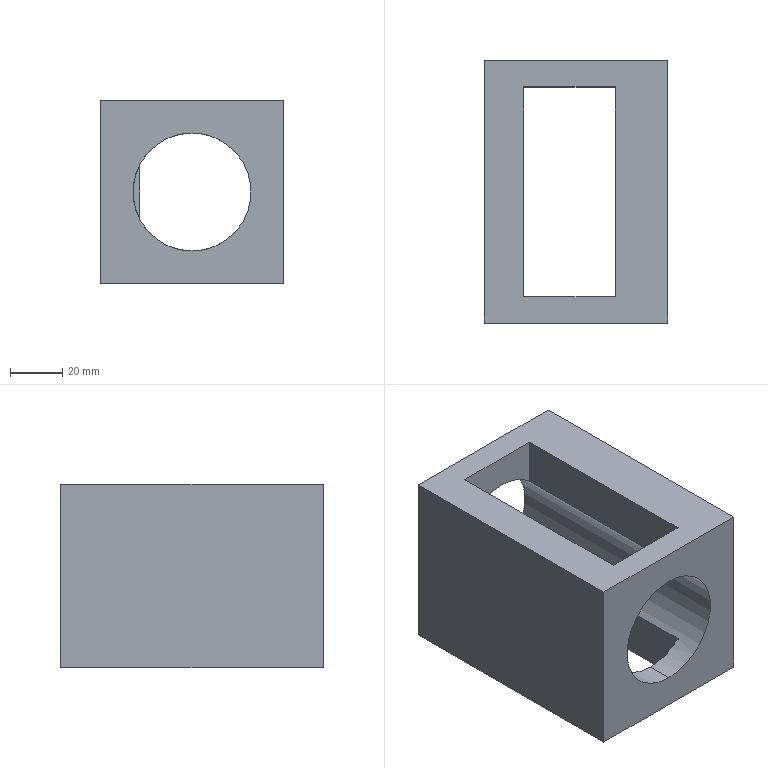Part | STEP file | Boss-Extrude 4 | 1 solid | 34 faces | box 70 x 100 x 70 mm | volume 247035 mm3 | plane 15 | cylinder 11 | cone 8 | commonest cylinder face diameters 5 x8 45 x3
STEP:
#1=CARTESIAN_POINT('',(-1518.738,1643.264,2784.251));
#2=VERTEX_POINT('',#1);
#3=CARTESIAN_POINT('',(-1518.738,1643.264,2789.251));
#4=VERTEX_POINT('',#3);
#5=CARTESIAN_POINT('',(-1518.738,1643.264,2786.751));
#6=DIRECTION('',(0.,1.,0.));
#7=DIRECTION('',(0.,0.,1.));
#8=AXIS2_PLACEMENT_3D('',#5,#6,#7);
#9=CIRCLE('',#8,2.5);
#10=EDGE_CURVE('',#2,#4,#9,.T.);
#11=ORIENTED_EDGE('',*,*,#10,.F.);
#12=CARTESIAN_POINT('',(-1518.738,1658.264,2784.251));
#13=VERTEX_POINT('',#12);
#14=CARTESIAN_POINT('',(-1518.738,1658.264,2784.251));
#15=DIRECTION('',(0.,1.,0.));
#16=VECTOR('',#15,1000.);
#17=LINE('',#14,#16);
#18=EDGE_CURVE('',#2,#13,#17,.T.);
#19=ORIENTED_EDGE('',*,*,#18,.T.);
#20=CARTESIAN_POINT('',(-1518.738,1658.264,2789.251));
#21=VERTEX_POINT('',#20);
#22=CARTESIAN_POINT('',(-1518.738,1658.264,2786.751));
#23=DIRECTION('',(0.,1.,0.));
#24=DIRECTION('',(0.,0.,1.));
#25=AXIS2_PLACEMENT_3D('',#22,#23,#24);
#26=CIRCLE('',#25,2.5);
#27=EDGE_CURVE('',#13,#21,#26,.T.);
#28=ORIENTED_EDGE('',*,*,#27,.T.);
#29=CARTESIAN_POINT('',(-1518.738,1658.264,2789.251));
#30=DIRECTION('',(0.,1.,0.));
#31=VECTOR('',#30,1000.);
#32=LINE('',#29,#31);
#33=EDGE_CURVE('',#4,#21,#32,.T.);
#34=ORIENTED_EDGE('',*,*,#33,.F.);
#35=EDGE_LOOP('',(#11,#19,#28,#34));
#36=FACE_OUTER_BOUND('',#35,.T.);
#37=CARTESIAN_POINT('',(-1518.738,1658.264,2786.751));
#38=DIRECTION('',(0.,1.,0.));
#39=DIRECTION('',(0.,0.,-1.));
#40=AXIS2_PLACEMENT_3D('',#37,#38,#39);
#41=CYLINDRICAL_SURFACE('',#40,2.5);
#42=ADVANCED_FACE('',(#36),#41,.F.);
#43=CARTESIAN_POINT('',(-1518.738,1641.762,2786.751));
#44=VERTEX_POINT('',#43);
#45=CARTESIAN_POINT('',(-1518.738,1643.264,2789.251));
#46=DIRECTION('',(0.,0.515,0.8572));
#47=VECTOR('',#46,1000.);
#48=LINE('',#45,#47);
#49=EDGE_CURVE('',#44,#4,#48,.T.);
#50=ORIENTED_EDGE('',*,*,#49,.F.);
#51=CARTESIAN_POINT('',(-1518.738,1643.264,2784.251));
#52=DIRECTION('',(0.,0.515,-0.8572));
#53=VECTOR('',#52,1000.);
#54=LINE('',#51,#53);
#55=EDGE_CURVE('',#44,#2,#54,.T.);
#56=ORIENTED_EDGE('',*,*,#55,.T.);
#57=ORIENTED_EDGE('',*,*,#10,.T.);
#58=EDGE_LOOP('',(#50,#56,#57));
#59=FACE_OUTER_BOUND('',#58,.T.);
#60=CARTESIAN_POINT('',(-1518.738,1643.264,2786.751));
#61=DIRECTION('',(0.,1.,0.));
#62=DIRECTION('',(0.,0.,-1.));
#63=AXIS2_PLACEMENT_3D('',#60,#61,#62);
#64=CONICAL_SURFACE('',#63,2.5,1.03);
#65=ADVANCED_FACE('',(#59),#64,.F.);
#66=CARTESIAN_POINT('',(-1458.738,1643.264,2844.251));
#67=VERTEX_POINT('',#66);
#68=CARTESIAN_POINT('',(-1458.738,1643.264,2849.251));
#69=VERTEX_POINT('',#68);
#70=CARTESIAN_POINT('',(-1458.738,1643.264,2846.751));
#71=DIRECTION('',(0.,1.,0.));
#72=DIRECTION('',(0.,0.,1.));
#73=AXIS2_PLACEMENT_3D('',#70,#71,#72);
#74=CIRCLE('',#73,2.5);
#75=EDGE_CURVE('',#67,#69,#74,.T.);
#76=ORIENTED_EDGE('',*,*,#75,.F.);
#77=CARTESIAN_POINT('',(-1458.738,1658.264,2844.251));
#78=VERTEX_POINT('',#77);
#79=CARTESIAN_POINT('',(-1458.738,1658.264,2844.251));
#80=DIRECTION('',(0.,1.,0.));
#81=VECTOR('',#80,1000.);
#82=LINE('',#79,#81);
#83=EDGE_CURVE('',#67,#78,#82,.T.);
#84=ORIENTED_EDGE('',*,*,#83,.T.);
#85=CARTESIAN_POINT('',(-1458.738,1658.264,2849.251));
#86=VERTEX_POINT('',#85);
#87=CARTESIAN_POINT('',(-1458.738,1658.264,2846.751));
#88=DIRECTION('',(0.,1.,0.));
#89=DIRECTION('',(0.,0.,1.));
#90=AXIS2_PLACEMENT_3D('',#87,#88,#89);
#91=CIRCLE('',#90,2.5);
#92=EDGE_CURVE('',#78,#86,#91,.T.);
#93=ORIENTED_EDGE('',*,*,#92,.T.);
#94=CARTESIAN_POINT('',(-1458.738,1658.264,2849.251));
#95=DIRECTION('',(0.,1.,0.));
#96=VECTOR('',#95,1000.);
#97=LINE('',#94,#96);
#98=EDGE_CURVE('',#69,#86,#97,.T.);
#99=ORIENTED_EDGE('',*,*,#98,.F.);
#100=EDGE_LOOP('',(#76,#84,#93,#99));
#101=FACE_OUTER_BOUND('',#100,.T.);
#102=CARTESIAN_POINT('',(-1458.738,1658.264,2846.751));
#103=DIRECTION('',(0.,1.,0.));
#104=DIRECTION('',(0.,0.,-1.));
#105=AXIS2_PLACEMENT_3D('',#102,#103,#104);
#106=CYLINDRICAL_SURFACE('',#105,2.5);
#107=ADVANCED_FACE('',(#101),#106,.F.);
#108=CARTESIAN_POINT('',(-1458.738,1641.762,2846.751));
#109=VERTEX_POINT('',#108);
#110=CARTESIAN_POINT('',(-1458.738,1643.264,2849.251));
#111=DIRECTION('',(0.,0.515,0.8572));
#112=VECTOR('',#111,1000.);
#113=LINE('',#110,#112);
#114=EDGE_CURVE('',#109,#69,#113,.T.);
#115=ORIENTED_EDGE('',*,*,#114,.F.);
#116=CARTESIAN_POINT('',(-1458.738,1643.264,2844.251));
#117=DIRECTION('',(0.,0.515,-0.8572));
#118=VECTOR('',#117,1000.);
#119=LINE('',#116,#118);
#120=EDGE_CURVE('',#109,#67,#119,.T.);
#121=ORIENTED_EDGE('',*,*,#120,.T.);
#122=ORIENTED_EDGE('',*,*,#75,.T.);
#123=EDGE_LOOP('',(#115,#121,#122));
#124=FACE_OUTER_BOUND('',#123,.T.);
#125=CARTESIAN_POINT('',(-1458.738,1643.264,2846.751));
#126=DIRECTION('',(0.,1.,0.));
#127=DIRECTION('',(0.,0.,-1.));
#128=AXIS2_PLACEMENT_3D('',#125,#126,#127);
#129=CONICAL_SURFACE('',#128,2.5,1.03);
#130=ADVANCED_FACE('',(#124),#129,.F.);
#131=CARTESIAN_POINT('',(-1458.738,1643.264,2784.251));
#132=VERTEX_POINT('',#131);
#133=CARTESIAN_POINT('',(-1458.738,1643.264,2789.251));
#134=VERTEX_POINT('',#133);
#135=CARTESIAN_POINT('',(-1458.738,1643.264,2786.751));
#136=DIRECTION('',(0.,1.,0.));
#137=DIRECTION('',(0.,0.,1.));
#138=AXIS2_PLACEMENT_3D('',#135,#136,#137);
#139=CIRCLE('',#138,2.5);
#140=EDGE_CURVE('',#132,#134,#139,.T.);
#141=ORIENTED_EDGE('',*,*,#140,.F.);
#142=CARTESIAN_POINT('',(-1458.738,1658.264,2784.251));
#143=VERTEX_POINT('',#142);
#144=CARTESIAN_POINT('',(-1458.738,1658.264,2784.251));
#145=DIRECTION('',(0.,1.,0.));
#146=VECTOR('',#145,1000.);
#147=LINE('',#144,#146);
#148=EDGE_CURVE('',#132,#143,#147,.T.);
#149=ORIENTED_EDGE('',*,*,#148,.T.);
#150=CARTESIAN_POINT('',(-1458.738,1658.264,2789.251));
#151=VERTEX_POINT('',#150);
#152=CARTESIAN_POINT('',(-1458.738,1658.264,2786.751));
#153=DIRECTION('',(0.,1.,0.));
#154=DIRECTION('',(0.,0.,1.));
#155=AXIS2_PLACEMENT_3D('',#152,#153,#154);
#156=CIRCLE('',#155,2.5);
#157=EDGE_CURVE('',#143,#151,#156,.T.);
#158=ORIENTED_EDGE('',*,*,#157,.T.);
#159=CARTESIAN_POINT('',(-1458.738,1658.264,2789.251));
#160=DIRECTION('',(0.,1.,0.));
#161=VECTOR('',#160,1000.);
#162=LINE('',#159,#161);
#163=EDGE_CURVE('',#134,#151,#162,.T.);
#164=ORIENTED_EDGE('',*,*,#163,.F.);
#165=EDGE_LOOP('',(#141,#149,#158,#164));
#166=FACE_OUTER_BOUND('',#165,.T.);
#167=CARTESIAN_POINT('',(-1458.738,1658.264,2786.751));
#168=DIRECTION('',(0.,1.,0.));
#169=DIRECTION('',(0.,0.,-1.));
#170=AXIS2_PLACEMENT_3D('',#167,#168,#169);
#171=CYLINDRICAL_SURFACE('',#170,2.5);
#172=ADVANCED_FACE('',(#166),#171,.F.);
#173=CARTESIAN_POINT('',(-1458.738,1641.762,2786.751));
#174=VERTEX_POINT('',#173);
#175=CARTESIAN_POINT('',(-1458.738,1643.264,2789.251));
#176=DIRECTION('',(0.,0.515,0.8572));
#177=VECTOR('',#176,1000.);
#178=LINE('',#175,#177);
#179=EDGE_CURVE('',#174,#134,#178,.T.);
#180=ORIENTED_EDGE('',*,*,#179,.F.);
#181=CARTESIAN_POINT('',(-1458.738,1643.264,2784.251));
#182=DIRECTION('',(0.,0.515,-0.8572));
#183=VECTOR('',#182,1000.);
#184=LINE('',#181,#183);
#185=EDGE_CURVE('',#174,#132,#184,.T.);
#186=ORIENTED_EDGE('',*,*,#185,.T.);
#187=ORIENTED_EDGE('',*,*,#140,.T.);
#188=EDGE_LOOP('',(#180,#186,#187));
#189=FACE_OUTER_BOUND('',#188,.T.);
#190=CARTESIAN_POINT('',(-1458.738,1643.264,2786.751));
#191=DIRECTION('',(0.,1.,0.));
#192=DIRECTION('',(0.,0.,-1.));
#193=AXIS2_PLACEMENT_3D('',#190,#191,#192);
#194=CONICAL_SURFACE('',#193,2.5,1.03);
#195=ADVANCED_FACE('',(#189),#194,.F.);
#196=CARTESIAN_POINT('',(-1518.738,1643.264,2844.251));
#197=VERTEX_POINT('',#196);
#198=CARTESIAN_POINT('',(-1518.738,1643.264,2849.251));
#199=VERTEX_POINT('',#198);
#200=CARTESIAN_POINT('',(-1518.738,1643.264,2846.751));
#201=DIRECTION('',(0.,1.,0.));
#202=DIRECTION('',(0.,0.,1.));
#203=AXIS2_PLACEMENT_3D('',#200,#201,#202);
#204=CIRCLE('',#203,2.5);
#205=EDGE_CURVE('',#197,#199,#204,.T.);
#206=ORIENTED_EDGE('',*,*,#205,.F.);
#207=CARTESIAN_POINT('',(-1518.738,1658.264,2844.251));
#208=VERTEX_POINT('',#207);
#209=CARTESIAN_POINT('',(-1518.738,1658.264,2844.251));
#210=DIRECTION('',(0.,1.,0.));
#211=VECTOR('',#210,1000.);
#212=LINE('',#209,#211);
#213=EDGE_CURVE('',#197,#208,#212,.T.);
#214=ORIENTED_EDGE('',*,*,#213,.T.);
#215=CARTESIAN_POINT('',(-1518.738,1658.264,2849.251));
#216=VERTEX_POINT('',#215);
#217=CARTESIAN_POINT('',(-1518.738,1658.264,2846.751));
#218=DIRECTION('',(0.,1.,0.));
#219=DIRECTION('',(0.,0.,1.));
#220=AXIS2_PLACEMENT_3D('',#217,#218,#219);
#221=CIRCLE('',#220,2.5);
#222=EDGE_CURVE('',#208,#216,#221,.T.);
#223=ORIENTED_EDGE('',*,*,#222,.T.);
#224=CARTESIAN_POINT('',(-1518.738,1658.264,2849.251));
#225=DIRECTION('',(0.,1.,0.));
#226=VECTOR('',#225,1000.);
#227=LINE('',#224,#226);
#228=EDGE_CURVE('',#199,#216,#227,.T.);
#229=ORIENTED_EDGE('',*,*,#228,.F.);
#230=EDGE_LOOP('',(#206,#214,#223,#229));
#231=FACE_OUTER_BOUND('',#230,.T.);
#232=CARTESIAN_POINT('',(-1518.738,1658.264,2846.751));
#233=DIRECTION('',(0.,1.,0.));
#234=DIRECTION('',(0.,0.,-1.));
#235=AXIS2_PLACEMENT_3D('',#232,#233,#234);
#236=CYLINDRICAL_SURFACE('',#235,2.5);
#237=ADVANCED_FACE('',(#231),#236,.F.);
#238=CARTESIAN_POINT('',(-1518.738,1641.762,2846.751));
#239=VERTEX_POINT('',#238);
#240=CARTESIAN_POINT('',(-1518.738,1643.264,2849.251));
#241=DIRECTION('',(0.,0.515,0.8572));
#242=VECTOR('',#241,1000.);
#243=LINE('',#240,#242);
#244=EDGE_CURVE('',#239,#199,#243,.T.);
#245=ORIENTED_EDGE('',*,*,#244,.F.);
#246=CARTESIAN_POINT('',(-1518.738,1643.264,2844.251));
#247=DIRECTION('',(0.,0.515,-0.8572));
#248=VECTOR('',#247,1000.);
#249=LINE('',#246,#248);
#250=EDGE_CURVE('',#239,#197,#249,.T.);
#251=ORIENTED_EDGE('',*,*,#250,.T.);
#252=ORIENTED_EDGE('',*,*,#205,.T.);
#253=EDGE_LOOP('',(#245,#251,#252));
#254=FACE_OUTER_BOUND('',#253,.T.);
#255=CARTESIAN_POINT('',(-1518.738,1643.264,2846.751));
#256=DIRECTION('',(0.,1.,0.));
#257=DIRECTION('',(0.,0.,-1.));
#258=AXIS2_PLACEMENT_3D('',#255,#256,#257);
#259=CONICAL_SURFACE('',#258,2.5,1.03);
#260=ADVANCED_FACE('',(#254),#259,.F.);
#261=CARTESIAN_POINT('',(-1488.738,1558.264,2794.251));
#262=VERTEX_POINT('',#261);
#263=CARTESIAN_POINT('',(-1488.738,1558.264,2839.251));
#264=VERTEX_POINT('',#263);
#265=CARTESIAN_POINT('',(-1488.738,1558.264,2816.751));
#266=DIRECTION('',(0.,1.,0.));
#267=DIRECTION('',(0.,0.,1.));
#268=AXIS2_PLACEMENT_3D('',#265,#266,#267);
#269=CIRCLE('',#268,22.5);
#270=EDGE_CURVE('',#262,#264,#269,.T.);
#271=ORIENTED_EDGE('',*,*,#270,.F.);
#272=CARTESIAN_POINT('',(-1488.738,1568.264,2794.251));
#273=VERTEX_POINT('',#272);
#274=CARTESIAN_POINT('',(-1488.738,1541.264,2794.251));
#275=DIRECTION('',(0.,1.,0.));
#276=VECTOR('',#275,1000.);
#277=LINE('',#274,#276);
#278=EDGE_CURVE('',#262,#273,#277,.T.);
#279=ORIENTED_EDGE('',*,*,#278,.T.);
#280=CARTESIAN_POINT('',(-1508.738,1568.264,2806.443));
#281=VERTEX_POINT('',#280);
#282=CARTESIAN_POINT('',(-1488.738,1568.264,2816.751));
#283=DIRECTION('',(0.,-1.,0.));
#284=DIRECTION('',(0.,0.,-1.));
#285=AXIS2_PLACEMENT_3D('',#282,#283,#284);
#286=CIRCLE('',#285,22.5);
#287=EDGE_CURVE('',#281,#273,#286,.T.);
#288=ORIENTED_EDGE('',*,*,#287,.F.);
#289=CARTESIAN_POINT('',(-1508.738,1568.264,2827.058));
#290=VERTEX_POINT('',#289);
#291=CARTESIAN_POINT('',(-1488.738,1568.264,2816.751));
#292=DIRECTION('',(0.,-1.,0.));
#293=DIRECTION('',(0.,0.,-1.));
#294=AXIS2_PLACEMENT_3D('',#291,#292,#293);
#295=CIRCLE('',#294,22.5);
#296=EDGE_CURVE('',#290,#281,#295,.T.);
#297=ORIENTED_EDGE('',*,*,#296,.F.);
#298=CARTESIAN_POINT('',(-1488.738,1568.264,2839.251));
#299=VERTEX_POINT('',#298);
#300=CARTESIAN_POINT('',(-1488.738,1568.264,2816.751));
#301=DIRECTION('',(0.,-1.,0.));
#302=DIRECTION('',(0.,0.,-1.));
#303=AXIS2_PLACEMENT_3D('',#300,#301,#302);
#304=CIRCLE('',#303,22.5);
#305=EDGE_CURVE('',#299,#290,#304,.T.);
#306=ORIENTED_EDGE('',*,*,#305,.F.);
#307=CARTESIAN_POINT('',(-1488.738,1541.264,2839.251));
#308=DIRECTION('',(0.,1.,0.));
#309=VECTOR('',#308,1000.);
#310=LINE('',#307,#309);
#311=EDGE_CURVE('',#264,#299,#310,.T.);
#312=ORIENTED_EDGE('',*,*,#311,.F.);
#313=EDGE_LOOP('',(#271,#279,#288,#297,#306,#312));
#314=FACE_OUTER_BOUND('',#313,.T.);
#315=CARTESIAN_POINT('',(-1488.738,1541.264,2816.751));
#316=DIRECTION('',(0.,1.,0.));
#317=DIRECTION('',(0.,0.,-1.));
#318=AXIS2_PLACEMENT_3D('',#315,#316,#317);
#319=CYLINDRICAL_SURFACE('',#318,22.5);
#320=ADVANCED_FACE('',(#314),#319,.F.);
#321=CARTESIAN_POINT('',(-1488.738,1648.264,2794.251));
#322=VERTEX_POINT('',#321);
#323=CARTESIAN_POINT('',(-1508.738,1648.264,2806.443));
#324=VERTEX_POINT('',#323);
#325=CARTESIAN_POINT('',(-1488.738,1648.264,2816.751));
#326=DIRECTION('',(0.,1.,0.));
#327=DIRECTION('',(0.,0.,1.));
#328=AXIS2_PLACEMENT_3D('',#325,#326,#327);
#329=CIRCLE('',#328,22.5);
#330=EDGE_CURVE('',#322,#324,#329,.T.);
#331=ORIENTED_EDGE('',*,*,#330,.F.);
#332=CARTESIAN_POINT('',(-1488.738,1658.264,2794.251));
#333=VERTEX_POINT('',#332);
#334=CARTESIAN_POINT('',(-1488.738,1541.264,2794.251));
#335=DIRECTION('',(0.,1.,0.));
#336=VECTOR('',#335,1000.);
#337=LINE('',#334,#336);
#338=EDGE_CURVE('',#322,#333,#337,.T.);
#339=ORIENTED_EDGE('',*,*,#338,.T.);
#340=CARTESIAN_POINT('',(-1488.738,1658.264,2839.251));
#341=VERTEX_POINT('',#340);
#342=CARTESIAN_POINT('',(-1488.738,1658.264,2816.751));
#343=DIRECTION('',(0.,1.,0.));
#344=DIRECTION('',(0.,0.,1.));
#345=AXIS2_PLACEMENT_3D('',#342,#343,#344);
#346=CIRCLE('',#345,22.5);
#347=EDGE_CURVE('',#333,#341,#346,.T.);
#348=ORIENTED_EDGE('',*,*,#347,.T.);
#349=CARTESIAN_POINT('',(-1488.738,1648.264,2839.251));
#350=VERTEX_POINT('',#349);
#351=CARTESIAN_POINT('',(-1488.738,1541.264,2839.251));
#352=DIRECTION('',(0.,1.,0.));
#353=VECTOR('',#352,1000.);
#354=LINE('',#351,#353);
#355=EDGE_CURVE('',#350,#341,#354,.T.);
#356=ORIENTED_EDGE('',*,*,#355,.F.);
#357=CARTESIAN_POINT('',(-1508.738,1648.264,2827.058));
#358=VERTEX_POINT('',#357);
#359=CARTESIAN_POINT('',(-1488.738,1648.264,2816.751));
#360=DIRECTION('',(0.,1.,0.));
#361=DIRECTION('',(0.,0.,1.));
#362=AXIS2_PLACEMENT_3D('',#359,#360,#361);
#363=CIRCLE('',#362,22.5);
#364=EDGE_CURVE('',#358,#350,#363,.T.);
#365=ORIENTED_EDGE('',*,*,#364,.F.);
#366=CARTESIAN_POINT('',(-1488.738,1648.264,2816.751));
#367=DIRECTION('',(0.,1.,0.));
#368=DIRECTION('',(0.,0.,1.));
#369=AXIS2_PLACEMENT_3D('',#366,#367,#368);
#370=CIRCLE('',#369,22.5);
#371=EDGE_CURVE('',#324,#358,#370,.T.);
#372=ORIENTED_EDGE('',*,*,#371,.F.);
#373=EDGE_LOOP('',(#331,#339,#348,#356,#365,#372));
#374=FACE_OUTER_BOUND('',#373,.T.);
#375=CARTESIAN_POINT('',(-1488.738,1541.264,2816.751));
#376=DIRECTION('',(0.,1.,0.));
#377=DIRECTION('',(0.,0.,-1.));
#378=AXIS2_PLACEMENT_3D('',#375,#376,#377);
#379=CYLINDRICAL_SURFACE('',#378,22.5);
#380=ADVANCED_FACE('',(#374),#379,.F.);
#381=CARTESIAN_POINT('',(-1473.738,1648.264,2799.98));
#382=VERTEX_POINT('',#381);
#383=CARTESIAN_POINT('',(-1488.738,1648.264,2816.751));
#384=DIRECTION('',(0.,1.,0.));
#385=DIRECTION('',(0.,0.,1.));
#386=AXIS2_PLACEMENT_3D('',#383,#384,#385);
#387=CIRCLE('',#386,22.5);
#388=EDGE_CURVE('',#382,#322,#387,.T.);
#389=ORIENTED_EDGE('',*,*,#388,.T.);
#390=ORIENTED_EDGE('',*,*,#330,.T.);
#391=CARTESIAN_POINT('',(-1508.738,1648.264,2781.751));
#392=VERTEX_POINT('',#391);
#393=CARTESIAN_POINT('',(-1508.738,1648.264,2881.751));
#394=DIRECTION('',(0.,0.,-1.));
#395=VECTOR('',#394,1000.);
#396=LINE('',#393,#395);
#397=EDGE_CURVE('',#324,#392,#396,.T.);
#398=ORIENTED_EDGE('',*,*,#397,.T.);
#399=CARTESIAN_POINT('',(-1473.738,1648.264,2781.751));
#400=VERTEX_POINT('',#399);
#401=CARTESIAN_POINT('',(-1468.738,1648.264,2781.751));
#402=DIRECTION('',(1.,0.,0.));
#403=VECTOR('',#402,1000.);
#404=LINE('',#401,#403);
#405=EDGE_CURVE('',#392,#400,#404,.T.);
#406=ORIENTED_EDGE('',*,*,#405,.T.);
#407=CARTESIAN_POINT('',(-1473.738,1648.264,2931.907));
#408=DIRECTION('',(0.,0.,-1.));
#409=VECTOR('',#408,1000.);
#410=LINE('',#407,#409);
#411=EDGE_CURVE('',#382,#400,#410,.T.);
#412=ORIENTED_EDGE('',*,*,#411,.F.);
#413=EDGE_LOOP('',(#389,#390,#398,#406,#412));
#414=FACE_OUTER_BOUND('',#413,.T.);
#415=CARTESIAN_POINT('',(-1468.738,1648.264,2881.751));
#416=DIRECTION('',(0.,1.,0.));
#417=DIRECTION('',(0.,0.,-1.));
#418=AXIS2_PLACEMENT_3D('',#415,#416,#417);
#419=PLANE('',#418);
#420=ADVANCED_FACE('',(#414),#419,.F.);
#421=CARTESIAN_POINT('',(-1508.738,1648.264,2851.751));
#422=VERTEX_POINT('',#421);
#423=CARTESIAN_POINT('',(-1508.738,1648.264,2881.751));
#424=DIRECTION('',(0.,0.,-1.));
#425=VECTOR('',#424,1000.);
#426=LINE('',#423,#425);
#427=EDGE_CURVE('',#422,#358,#426,.T.);
#428=ORIENTED_EDGE('',*,*,#427,.T.);
#429=ORIENTED_EDGE('',*,*,#364,.T.);
#430=CARTESIAN_POINT('',(-1473.738,1648.264,2833.521));
#431=VERTEX_POINT('',#430);
#432=CARTESIAN_POINT('',(-1488.738,1648.264,2816.751));
#433=DIRECTION('',(0.,1.,0.));
#434=DIRECTION('',(0.,0.,1.));
#435=AXIS2_PLACEMENT_3D('',#432,#433,#434);
#436=CIRCLE('',#435,22.5);
#437=EDGE_CURVE('',#350,#431,#436,.T.);
#438=ORIENTED_EDGE('',*,*,#437,.T.);
#439=CARTESIAN_POINT('',(-1473.738,1648.264,2851.751));
#440=VERTEX_POINT('',#439);
#441=CARTESIAN_POINT('',(-1473.738,1648.264,2931.907));
#442=DIRECTION('',(0.,0.,-1.));
#443=VECTOR('',#442,1000.);
#444=LINE('',#441,#443);
#445=EDGE_CURVE('',#440,#431,#444,.T.);
#446=ORIENTED_EDGE('',*,*,#445,.F.);
#447=CARTESIAN_POINT('',(-1523.738,1648.264,2851.751));
#448=DIRECTION('',(1.,0.,0.));
#449=VECTOR('',#448,1000.);
#450=LINE('',#447,#449);
#451=EDGE_CURVE('',#422,#440,#450,.T.);
#452=ORIENTED_EDGE('',*,*,#451,.F.);
#453=EDGE_LOOP('',(#428,#429,#438,#446,#452));
#454=FACE_OUTER_BOUND('',#453,.T.);
#455=CARTESIAN_POINT('',(-1468.738,1648.264,2881.751));
#456=DIRECTION('',(0.,1.,0.));
#457=DIRECTION('',(0.,0.,-1.));
#458=AXIS2_PLACEMENT_3D('',#455,#456,#457);
#459=PLANE('',#458);
#460=ADVANCED_FACE('',(#454),#459,.F.);
#461=CARTESIAN_POINT('',(-1473.738,1568.264,2833.521));
#462=VERTEX_POINT('',#461);
#463=CARTESIAN_POINT('',(-1488.738,1568.264,2816.751));
#464=DIRECTION('',(0.,-1.,0.));
#465=DIRECTION('',(0.,0.,-1.));
#466=AXIS2_PLACEMENT_3D('',#463,#464,#465);
#467=CIRCLE('',#466,22.5);
#468=EDGE_CURVE('',#462,#299,#467,.T.);
#469=ORIENTED_EDGE('',*,*,#468,.T.);
#470=ORIENTED_EDGE('',*,*,#305,.T.);
#471=CARTESIAN_POINT('',(-1508.738,1568.264,2851.751));
#472=VERTEX_POINT('',#471);
#473=CARTESIAN_POINT('',(-1508.738,1568.264,2881.751));
#474=DIRECTION('',(0.,0.,-1.));
#475=VECTOR('',#474,1000.);
#476=LINE('',#473,#475);
#477=EDGE_CURVE('',#472,#290,#476,.T.);
#478=ORIENTED_EDGE('',*,*,#477,.F.);
#479=CARTESIAN_POINT('',(-1473.738,1568.264,2851.751));
#480=VERTEX_POINT('',#479);
#481=CARTESIAN_POINT('',(-1523.738,1568.264,2851.751));
#482=DIRECTION('',(-1.,0.,0.));
#483=VECTOR('',#482,1000.);
#484=LINE('',#481,#483);
#485=EDGE_CURVE('',#480,#472,#484,.T.);
#486=ORIENTED_EDGE('',*,*,#485,.F.);
#487=CARTESIAN_POINT('',(-1473.738,1568.264,2931.907));
#488=DIRECTION('',(0.,0.,-1.));
#489=VECTOR('',#488,1000.);
#490=LINE('',#487,#489);
#491=EDGE_CURVE('',#480,#462,#490,.T.);
#492=ORIENTED_EDGE('',*,*,#491,.T.);
#493=EDGE_LOOP('',(#469,#470,#478,#486,#492));
#494=FACE_OUTER_BOUND('',#493,.T.);
#495=CARTESIAN_POINT('',(-1468.738,1568.264,2881.751));
#496=DIRECTION('',(0.,-1.,0.));
#497=DIRECTION('',(0.,0.,1.));
#498=AXIS2_PLACEMENT_3D('',#495,#496,#497);
#499=PLANE('',#498);
#500=ADVANCED_FACE('',(#494),#499,.F.);
#501=CARTESIAN_POINT('',(-1508.738,1568.264,2781.751));
#502=VERTEX_POINT('',#501);
#503=CARTESIAN_POINT('',(-1508.738,1568.264,2881.751));
#504=DIRECTION('',(0.,0.,-1.));
#505=VECTOR('',#504,1000.);
#506=LINE('',#503,#505);
#507=EDGE_CURVE('',#281,#502,#506,.T.);
#508=ORIENTED_EDGE('',*,*,#507,.F.);
#509=ORIENTED_EDGE('',*,*,#287,.T.);
#510=CARTESIAN_POINT('',(-1473.738,1568.264,2799.98));
#511=VERTEX_POINT('',#510);
#512=CARTESIAN_POINT('',(-1488.738,1568.264,2816.751));
#513=DIRECTION('',(0.,-1.,0.));
#514=DIRECTION('',(0.,0.,-1.));
#515=AXIS2_PLACEMENT_3D('',#512,#513,#514);
#516=CIRCLE('',#515,22.5);
#517=EDGE_CURVE('',#273,#511,#516,.T.);
#518=ORIENTED_EDGE('',*,*,#517,.T.);
#519=CARTESIAN_POINT('',(-1473.738,1568.264,2781.751));
#520=VERTEX_POINT('',#519);
#521=CARTESIAN_POINT('',(-1473.738,1568.264,2931.907));
#522=DIRECTION('',(0.,0.,-1.));
#523=VECTOR('',#522,1000.);
#524=LINE('',#521,#523);
#525=EDGE_CURVE('',#511,#520,#524,.T.);
#526=ORIENTED_EDGE('',*,*,#525,.T.);
#527=CARTESIAN_POINT('',(-1468.738,1568.264,2781.751));
#528=DIRECTION('',(-1.,0.,0.));
#529=VECTOR('',#528,1000.);
#530=LINE('',#527,#529);
#531=EDGE_CURVE('',#520,#502,#530,.T.);
#532=ORIENTED_EDGE('',*,*,#531,.T.);
#533=EDGE_LOOP('',(#508,#509,#518,#526,#532));
#534=FACE_OUTER_BOUND('',#533,.T.);
#535=CARTESIAN_POINT('',(-1468.738,1568.264,2881.751));
#536=DIRECTION('',(0.,-1.,0.));
#537=DIRECTION('',(0.,0.,1.));
#538=AXIS2_PLACEMENT_3D('',#535,#536,#537);
#539=PLANE('',#538);
#540=ADVANCED_FACE('',(#534),#539,.F.);
#541=CARTESIAN_POINT('',(-1473.738,1541.264,2833.521));
#542=DIRECTION('',(0.,1.,0.));
#543=VECTOR('',#542,1000.);
#544=LINE('',#541,#543);
#545=EDGE_CURVE('',#462,#431,#544,.T.);
#546=ORIENTED_EDGE('',*,*,#545,.F.);
#547=ORIENTED_EDGE('',*,*,#491,.F.);
#548=CARTESIAN_POINT('',(-1473.738,1648.264,2851.751));
#549=DIRECTION('',(0.,-1.,0.));
#550=VECTOR('',#549,1000.);
#551=LINE('',#548,#550);
#552=EDGE_CURVE('',#440,#480,#551,.T.);
#553=ORIENTED_EDGE('',*,*,#552,.F.);
#554=ORIENTED_EDGE('',*,*,#445,.T.);
#555=EDGE_LOOP('',(#546,#547,#553,#554));
#556=FACE_OUTER_BOUND('',#555,.T.);
#557=CARTESIAN_POINT('',(-1473.738,1648.264,2931.907));
#558=DIRECTION('',(-1.,0.,0.));
#559=DIRECTION('',(0.,1.,0.));
#560=AXIS2_PLACEMENT_3D('',#557,#558,#559);
#561=PLANE('',#560);
#562=ADVANCED_FACE('',(#556),#561,.T.);
#563=CARTESIAN_POINT('',(-1453.738,1558.264,2851.751));
#564=VERTEX_POINT('',#563);
#565=CARTESIAN_POINT('',(-1453.738,1558.264,2781.751));
#566=VERTEX_POINT('',#565);
#567=CARTESIAN_POINT('',(-1453.738,1558.264,2781.751));
#568=DIRECTION('',(0.,0.,-1.));
#569=VECTOR('',#568,1000.);
#570=LINE('',#567,#569);
#571=EDGE_CURVE('',#564,#566,#570,.T.);
#572=ORIENTED_EDGE('',*,*,#571,.T.);
#573=CARTESIAN_POINT('',(-1453.738,1658.264,2781.751));
#574=VERTEX_POINT('',#573);
#575=CARTESIAN_POINT('',(-1453.738,1658.264,2781.751));
#576=DIRECTION('',(0.,-1.,0.));
#577=VECTOR('',#576,1000.);
#578=LINE('',#575,#577);
#579=EDGE_CURVE('',#574,#566,#578,.T.);
#580=ORIENTED_EDGE('',*,*,#579,.F.);
#581=CARTESIAN_POINT('',(-1453.738,1658.264,2851.751));
#582=VERTEX_POINT('',#581);
#583=CARTESIAN_POINT('',(-1453.738,1658.264,2781.751));
#584=DIRECTION('',(0.,0.,-1.));
#585=VECTOR('',#584,1000.);
#586=LINE('',#583,#585);
#587=EDGE_CURVE('',#582,#574,#586,.T.);
#588=ORIENTED_EDGE('',*,*,#587,.F.);
#589=CARTESIAN_POINT('',(-1453.738,1658.264,2851.751));
#590=DIRECTION('',(0.,-1.,0.));
#591=VECTOR('',#590,1000.);
#592=LINE('',#589,#591);
#593=EDGE_CURVE('',#582,#564,#592,.T.);
#594=ORIENTED_EDGE('',*,*,#593,.T.);
#595=EDGE_LOOP('',(#572,#580,#588,#594));
#596=FACE_OUTER_BOUND('',#595,.T.);
#597=CARTESIAN_POINT('',(-1453.738,1658.264,2781.751));
#598=DIRECTION('',(-1.,0.,0.));
#599=DIRECTION('',(0.,0.,-1.));
#600=AXIS2_PLACEMENT_3D('',#597,#598,#599);
#601=PLANE('',#600);
#602=ADVANCED_FACE('',(#596),#601,.F.);
#603=ORIENTED_EDGE('',*,*,#531,.F.);
#604=CARTESIAN_POINT('',(-1473.738,1648.264,2781.751));
#605=DIRECTION('',(0.,1.,0.));
#606=VECTOR('',#605,1000.);
#607=LINE('',#604,#606);
#608=EDGE_CURVE('',#520,#400,#607,.T.);
#609=ORIENTED_EDGE('',*,*,#608,.T.);
#610=ORIENTED_EDGE('',*,*,#405,.F.);
#611=CARTESIAN_POINT('',(-1508.738,1648.264,2781.751));
#612=DIRECTION('',(0.,1.,0.));
#613=VECTOR('',#612,1000.);
#614=LINE('',#611,#613);
#615=EDGE_CURVE('',#502,#392,#614,.T.);
#616=ORIENTED_EDGE('',*,*,#615,.F.);
#617=EDGE_LOOP('',(#603,#609,#610,#616));
#618=FACE_BOUND('',#617,.T.);
#619=CARTESIAN_POINT('',(-1523.738,1558.264,2781.751));
#620=VERTEX_POINT('',#619);
#621=CARTESIAN_POINT('',(-1523.738,1558.264,2781.751));
#622=DIRECTION('',(-1.,0.,0.));
#623=VECTOR('',#622,1000.);
#624=LINE('',#621,#623);
#625=EDGE_CURVE('',#566,#620,#624,.T.);
#626=ORIENTED_EDGE('',*,*,#625,.T.);
#627=CARTESIAN_POINT('',(-1523.738,1658.264,2781.751));
#628=VERTEX_POINT('',#627);
#629=CARTESIAN_POINT('',(-1523.738,1658.264,2781.751));
#630=DIRECTION('',(0.,-1.,0.));
#631=VECTOR('',#630,1000.);
#632=LINE('',#629,#631);
#633=EDGE_CURVE('',#628,#620,#632,.T.);
#634=ORIENTED_EDGE('',*,*,#633,.F.);
#635=CARTESIAN_POINT('',(-1523.738,1658.264,2781.751));
#636=DIRECTION('',(-1.,0.,0.));
#637=VECTOR('',#636,1000.);
#638=LINE('',#635,#637);
#639=EDGE_CURVE('',#574,#628,#638,.T.);
#640=ORIENTED_EDGE('',*,*,#639,.F.);
#641=ORIENTED_EDGE('',*,*,#579,.T.);
#642=EDGE_LOOP('',(#626,#634,#640,#641));
#643=FACE_OUTER_BOUND('',#642,.T.);
#644=CARTESIAN_POINT('',(-1523.738,1658.264,2781.751));
#645=DIRECTION('',(0.,0.,1.));
#646=DIRECTION('',(-1.,0.,0.));
#647=AXIS2_PLACEMENT_3D('',#644,#645,#646);
#648=PLANE('',#647);
#649=ADVANCED_FACE('',(#618,#643),#648,.F.);
#650=CARTESIAN_POINT('',(-1523.738,1558.264,2851.751));
#651=VERTEX_POINT('',#650);
#652=CARTESIAN_POINT('',(-1523.738,1558.264,2781.751));
#653=DIRECTION('',(0.,0.,1.));
#654=VECTOR('',#653,1000.);
#655=LINE('',#652,#654);
#656=EDGE_CURVE('',#620,#651,#655,.T.);
#657=ORIENTED_EDGE('',*,*,#656,.T.);
#658=CARTESIAN_POINT('',(-1523.738,1658.264,2851.751));
#659=VERTEX_POINT('',#658);
#660=CARTESIAN_POINT('',(-1523.738,1658.264,2851.751));
#661=DIRECTION('',(0.,-1.,0.));
#662=VECTOR('',#661,1000.);
#663=LINE('',#660,#662);
#664=EDGE_CURVE('',#659,#651,#663,.T.);
#665=ORIENTED_EDGE('',*,*,#664,.F.);
#666=CARTESIAN_POINT('',(-1523.738,1658.264,2781.751));
#667=DIRECTION('',(0.,0.,1.));
#668=VECTOR('',#667,1000.);
#669=LINE('',#666,#668);
#670=EDGE_CURVE('',#628,#659,#669,.T.);
#671=ORIENTED_EDGE('',*,*,#670,.F.);
#672=ORIENTED_EDGE('',*,*,#633,.T.);
#673=EDGE_LOOP('',(#657,#665,#671,#672));
#674=FACE_OUTER_BOUND('',#673,.T.);
#675=CARTESIAN_POINT('',(-1523.738,1658.264,2781.751));
#676=DIRECTION('',(1.,0.,0.));
#677=DIRECTION('',(0.,0.,1.));
#678=AXIS2_PLACEMENT_3D('',#675,#676,#677);
#679=PLANE('',#678);
#680=ADVANCED_FACE('',(#674),#679,.F.);
#681=ORIENTED_EDGE('',*,*,#451,.T.);
#682=ORIENTED_EDGE('',*,*,#552,.T.);
#683=ORIENTED_EDGE('',*,*,#485,.T.);
#684=CARTESIAN_POINT('',(-1508.738,1658.264,2851.751));
#685=DIRECTION('',(0.,1.,0.));
#686=VECTOR('',#685,1000.);
#687=LINE('',#684,#686);
#688=EDGE_CURVE('',#472,#422,#687,.T.);
#689=ORIENTED_EDGE('',*,*,#688,.T.);
#690=EDGE_LOOP('',(#681,#682,#683,#689));
#691=FACE_BOUND('',#690,.T.);
#692=CARTESIAN_POINT('',(-1523.738,1558.264,2851.751));
#693=DIRECTION('',(1.,0.,0.));
#694=VECTOR('',#693,1000.);
#695=LINE('',#692,#694);
#696=EDGE_CURVE('',#651,#564,#695,.T.);
#697=ORIENTED_EDGE('',*,*,#696,.T.);
#698=ORIENTED_EDGE('',*,*,#593,.F.);
#699=CARTESIAN_POINT('',(-1523.738,1658.264,2851.751));
#700=DIRECTION('',(1.,0.,0.));
#701=VECTOR('',#700,1000.);
#702=LINE('',#699,#701);
#703=EDGE_CURVE('',#659,#582,#702,.T.);
#704=ORIENTED_EDGE('',*,*,#703,.F.);
#705=ORIENTED_EDGE('',*,*,#664,.T.);
#706=EDGE_LOOP('',(#697,#698,#704,#705));
#707=FACE_OUTER_BOUND('',#706,.T.);
#708=CARTESIAN_POINT('',(-1523.738,1658.264,2851.751));
#709=DIRECTION('',(0.,0.,-1.));
#710=DIRECTION('',(1.,0.,0.));
#711=AXIS2_PLACEMENT_3D('',#708,#709,#710);
#712=PLANE('',#711);
#713=ADVANCED_FACE('',(#691,#707),#712,.F.);
#714=CARTESIAN_POINT('',(-1518.738,1658.264,2786.751));
#715=DIRECTION('',(0.,1.,0.));
#716=DIRECTION('',(0.,0.,1.));
#717=AXIS2_PLACEMENT_3D('',#714,#715,#716);
#718=CIRCLE('',#717,2.5);
#719=EDGE_CURVE('',#21,#13,#718,.T.);
#720=ORIENTED_EDGE('',*,*,#719,.F.);
#721=ORIENTED_EDGE('',*,*,#27,.F.);
#722=EDGE_LOOP('',(#720,#721));
#723=FACE_BOUND('',#722,.T.);
#724=CARTESIAN_POINT('',(-1458.738,1658.264,2846.751));
#725=DIRECTION('',(0.,1.,0.));
#726=DIRECTION('',(0.,0.,1.));
#727=AXIS2_PLACEMENT_3D('',#724,#725,#726);
#728=CIRCLE('',#727,2.5);
#729=EDGE_CURVE('',#86,#78,#728,.T.);
#730=ORIENTED_EDGE('',*,*,#729,.F.);
#731=ORIENTED_EDGE('',*,*,#92,.F.);
#732=EDGE_LOOP('',(#730,#731));
#733=FACE_BOUND('',#732,.T.);
#734=CARTESIAN_POINT('',(-1458.738,1658.264,2786.751));
#735=DIRECTION('',(0.,1.,0.));
#736=DIRECTION('',(0.,0.,1.));
#737=AXIS2_PLACEMENT_3D('',#734,#735,#736);
#738=CIRCLE('',#737,2.5);
#739=EDGE_CURVE('',#151,#143,#738,.T.);
#740=ORIENTED_EDGE('',*,*,#739,.F.);
#741=ORIENTED_EDGE('',*,*,#157,.F.);
#742=EDGE_LOOP('',(#740,#741));
#743=FACE_BOUND('',#742,.T.);
#744=CARTESIAN_POINT('',(-1518.738,1658.264,2846.751));
#745=DIRECTION('',(0.,1.,0.));
#746=DIRECTION('',(0.,0.,1.));
#747=AXIS2_PLACEMENT_3D('',#744,#745,#746);
#748=CIRCLE('',#747,2.5);
#749=EDGE_CURVE('',#216,#208,#748,.T.);
#750=ORIENTED_EDGE('',*,*,#749,.F.);
#751=ORIENTED_EDGE('',*,*,#222,.F.);
#752=EDGE_LOOP('',(#750,#751));
#753=FACE_BOUND('',#752,.T.);
#754=CARTESIAN_POINT('',(-1488.738,1658.264,2816.751));
#755=DIRECTION('',(0.,1.,0.));
#756=DIRECTION('',(0.,0.,1.));
#757=AXIS2_PLACEMENT_3D('',#754,#755,#756);
#758=CIRCLE('',#757,22.5);
#759=EDGE_CURVE('',#341,#333,#758,.T.);
#760=ORIENTED_EDGE('',*,*,#759,.F.);
#761=ORIENTED_EDGE('',*,*,#347,.F.);
#762=EDGE_LOOP('',(#760,#761));
#763=FACE_BOUND('',#762,.T.);
#764=ORIENTED_EDGE('',*,*,#587,.T.);
#765=ORIENTED_EDGE('',*,*,#639,.T.);
#766=ORIENTED_EDGE('',*,*,#670,.T.);
#767=ORIENTED_EDGE('',*,*,#703,.T.);
#768=EDGE_LOOP('',(#764,#765,#766,#767));
#769=FACE_OUTER_BOUND('',#768,.T.);
#770=CARTESIAN_POINT('',(-1488.738,1658.264,2816.751));
#771=DIRECTION('',(0.,1.,0.));
#772=DIRECTION('',(0.,0.,-1.));
#773=AXIS2_PLACEMENT_3D('',#770,#771,#772);
#774=PLANE('',#773);
#775=ADVANCED_FACE('',(#723,#733,#743,#753,#763,#769),#774,.T.);
#776=CARTESIAN_POINT('',(-1488.738,1558.264,2816.751));
#777=DIRECTION('',(0.,1.,0.));
#778=DIRECTION('',(0.,0.,1.));
#779=AXIS2_PLACEMENT_3D('',#776,#777,#778);
#780=CIRCLE('',#779,22.5);
#781=EDGE_CURVE('',#264,#262,#780,.T.);
#782=ORIENTED_EDGE('',*,*,#781,.T.);
#783=ORIENTED_EDGE('',*,*,#270,.T.);
#784=EDGE_LOOP('',(#782,#783));
#785=FACE_BOUND('',#784,.T.);
#786=ORIENTED_EDGE('',*,*,#571,.F.);
#787=ORIENTED_EDGE('',*,*,#696,.F.);
#788=ORIENTED_EDGE('',*,*,#656,.F.);
#789=ORIENTED_EDGE('',*,*,#625,.F.);
#790=EDGE_LOOP('',(#786,#787,#788,#789));
#791=FACE_OUTER_BOUND('',#790,.T.);
#792=CARTESIAN_POINT('',(-1488.738,1558.264,2816.751));
#793=DIRECTION('',(0.,1.,0.));
#794=DIRECTION('',(0.,0.,-1.));
#795=AXIS2_PLACEMENT_3D('',#792,#793,#794);
#796=PLANE('',#795);
#797=ADVANCED_FACE('',(#785,#791),#796,.F.);
#798=ORIENTED_EDGE('',*,*,#397,.F.);
#799=CARTESIAN_POINT('',(-1508.738,1648.264,2796.751));
#800=DIRECTION('',(0.,0.,1.));
#801=VECTOR('',#800,1000.);
#802=LINE('',#799,#801);
#803=EDGE_CURVE('',#324,#358,#802,.T.);
#804=ORIENTED_EDGE('',*,*,#803,.T.);
#805=ORIENTED_EDGE('',*,*,#427,.F.);
#806=ORIENTED_EDGE('',*,*,#688,.F.);
#807=ORIENTED_EDGE('',*,*,#477,.T.);
#808=CARTESIAN_POINT('',(-1508.738,1568.264,2796.751));
#809=DIRECTION('',(0.,0.,-1.));
#810=VECTOR('',#809,1000.);
#811=LINE('',#808,#810);
#812=EDGE_CURVE('',#290,#281,#811,.T.);
#813=ORIENTED_EDGE('',*,*,#812,.T.);
#814=ORIENTED_EDGE('',*,*,#507,.T.);
#815=ORIENTED_EDGE('',*,*,#615,.T.);
#816=EDGE_LOOP('',(#798,#804,#805,#806,#807,#813,#814,#815));
#817=FACE_OUTER_BOUND('',#816,.T.);
#818=CARTESIAN_POINT('',(-1508.738,1648.264,2881.751));
#819=DIRECTION('',(-1.,0.,0.));
#820=DIRECTION('',(0.,0.,-1.));
#821=AXIS2_PLACEMENT_3D('',#818,#819,#820);
#822=PLANE('',#821);
#823=ADVANCED_FACE('',(#817),#822,.F.);
#824=CARTESIAN_POINT('',(-1473.738,1541.264,2799.98));
#825=DIRECTION('',(0.,-1.,0.));
#826=VECTOR('',#825,1000.);
#827=LINE('',#824,#826);
#828=EDGE_CURVE('',#382,#511,#827,.T.);
#829=ORIENTED_EDGE('',*,*,#828,.F.);
#830=ORIENTED_EDGE('',*,*,#411,.T.);
#831=ORIENTED_EDGE('',*,*,#608,.F.);
#832=ORIENTED_EDGE('',*,*,#525,.F.);
#833=EDGE_LOOP('',(#829,#830,#831,#832));
#834=FACE_OUTER_BOUND('',#833,.T.);
#835=CARTESIAN_POINT('',(-1473.738,1648.264,2931.907));
#836=DIRECTION('',(-1.,0.,0.));
#837=DIRECTION('',(0.,1.,0.));
#838=AXIS2_PLACEMENT_3D('',#835,#836,#837);
#839=PLANE('',#838);
#840=ADVANCED_FACE('',(#834),#839,.T.);
#841=ORIENTED_EDGE('',*,*,#278,.F.);
#842=ORIENTED_EDGE('',*,*,#781,.F.);
#843=ORIENTED_EDGE('',*,*,#311,.T.);
#844=ORIENTED_EDGE('',*,*,#468,.F.);
#845=ORIENTED_EDGE('',*,*,#545,.T.);
#846=ORIENTED_EDGE('',*,*,#437,.F.);
#847=ORIENTED_EDGE('',*,*,#355,.T.);
#848=ORIENTED_EDGE('',*,*,#759,.T.);
#849=ORIENTED_EDGE('',*,*,#338,.F.);
#850=ORIENTED_EDGE('',*,*,#388,.F.);
#851=ORIENTED_EDGE('',*,*,#828,.T.);
#852=ORIENTED_EDGE('',*,*,#517,.F.);
#853=EDGE_LOOP('',(#841,#842,#843,#844,#845,#846,#847,#848,#849,#850,#851,#852));
#854=FACE_OUTER_BOUND('',#853,.T.);
#855=CARTESIAN_POINT('',(-1488.738,1541.264,2816.751));
#856=DIRECTION('',(0.,1.,0.));
#857=DIRECTION('',(0.,0.,-1.));
#858=AXIS2_PLACEMENT_3D('',#855,#856,#857);
#859=CYLINDRICAL_SURFACE('',#858,22.5);
#860=ADVANCED_FACE('',(#854),#859,.F.);
#861=ORIENTED_EDGE('',*,*,#250,.F.);
#862=ORIENTED_EDGE('',*,*,#244,.T.);
#863=CARTESIAN_POINT('',(-1518.738,1643.264,2846.751));
#864=DIRECTION('',(0.,1.,0.));
#865=DIRECTION('',(0.,0.,1.));
#866=AXIS2_PLACEMENT_3D('',#863,#864,#865);
#867=CIRCLE('',#866,2.5);
#868=EDGE_CURVE('',#199,#197,#867,.T.);
#869=ORIENTED_EDGE('',*,*,#868,.T.);
#870=EDGE_LOOP('',(#861,#862,#869));
#871=FACE_OUTER_BOUND('',#870,.T.);
#872=CARTESIAN_POINT('',(-1518.738,1643.264,2846.751));
#873=DIRECTION('',(0.,1.,0.));
#874=DIRECTION('',(0.,0.,-1.));
#875=AXIS2_PLACEMENT_3D('',#872,#873,#874);
#876=CONICAL_SURFACE('',#875,2.5,1.03);
#877=ADVANCED_FACE('',(#871),#876,.F.);
#878=ORIENTED_EDGE('',*,*,#213,.F.);
#879=ORIENTED_EDGE('',*,*,#868,.F.);
#880=ORIENTED_EDGE('',*,*,#228,.T.);
#881=ORIENTED_EDGE('',*,*,#749,.T.);
#882=EDGE_LOOP('',(#878,#879,#880,#881));
#883=FACE_OUTER_BOUND('',#882,.T.);
#884=CARTESIAN_POINT('',(-1518.738,1658.264,2846.751));
#885=DIRECTION('',(0.,1.,0.));
#886=DIRECTION('',(0.,0.,-1.));
#887=AXIS2_PLACEMENT_3D('',#884,#885,#886);
#888=CYLINDRICAL_SURFACE('',#887,2.5);
#889=ADVANCED_FACE('',(#883),#888,.F.);
#890=ORIENTED_EDGE('',*,*,#185,.F.);
#891=ORIENTED_EDGE('',*,*,#179,.T.);
#892=CARTESIAN_POINT('',(-1458.738,1643.264,2786.751));
#893=DIRECTION('',(0.,1.,0.));
#894=DIRECTION('',(0.,0.,1.));
#895=AXIS2_PLACEMENT_3D('',#892,#893,#894);
#896=CIRCLE('',#895,2.5);
#897=EDGE_CURVE('',#134,#132,#896,.T.);
#898=ORIENTED_EDGE('',*,*,#897,.T.);
#899=EDGE_LOOP('',(#890,#891,#898));
#900=FACE_OUTER_BOUND('',#899,.T.);
#901=CARTESIAN_POINT('',(-1458.738,1643.264,2786.751));
#902=DIRECTION('',(0.,1.,0.));
#903=DIRECTION('',(0.,0.,-1.));
#904=AXIS2_PLACEMENT_3D('',#901,#902,#903);
#905=CONICAL_SURFACE('',#904,2.5,1.03);
#906=ADVANCED_FACE('',(#900),#905,.F.);
#907=ORIENTED_EDGE('',*,*,#148,.F.);
#908=ORIENTED_EDGE('',*,*,#897,.F.);
#909=ORIENTED_EDGE('',*,*,#163,.T.);
#910=ORIENTED_EDGE('',*,*,#739,.T.);
#911=EDGE_LOOP('',(#907,#908,#909,#910));
#912=FACE_OUTER_BOUND('',#911,.T.);
#913=CARTESIAN_POINT('',(-1458.738,1658.264,2786.751));
#914=DIRECTION('',(0.,1.,0.));
#915=DIRECTION('',(0.,0.,-1.));
#916=AXIS2_PLACEMENT_3D('',#913,#914,#915);
#917=CYLINDRICAL_SURFACE('',#916,2.5);
#918=ADVANCED_FACE('',(#912),#917,.F.);
#919=ORIENTED_EDGE('',*,*,#120,.F.);
#920=ORIENTED_EDGE('',*,*,#114,.T.);
#921=CARTESIAN_POINT('',(-1458.738,1643.264,2846.751));
#922=DIRECTION('',(0.,1.,0.));
#923=DIRECTION('',(0.,0.,1.));
#924=AXIS2_PLACEMENT_3D('',#921,#922,#923);
#925=CIRCLE('',#924,2.5);
#926=EDGE_CURVE('',#69,#67,#925,.T.);
#927=ORIENTED_EDGE('',*,*,#926,.T.);
#928=EDGE_LOOP('',(#919,#920,#927));
#929=FACE_OUTER_BOUND('',#928,.T.);
#930=CARTESIAN_POINT('',(-1458.738,1643.264,2846.751));
#931=DIRECTION('',(0.,1.,0.));
#932=DIRECTION('',(0.,0.,-1.));
#933=AXIS2_PLACEMENT_3D('',#930,#931,#932);
#934=CONICAL_SURFACE('',#933,2.5,1.03);
#935=ADVANCED_FACE('',(#929),#934,.F.);
#936=ORIENTED_EDGE('',*,*,#83,.F.);
#937=ORIENTED_EDGE('',*,*,#926,.F.);
#938=ORIENTED_EDGE('',*,*,#98,.T.);
#939=ORIENTED_EDGE('',*,*,#729,.T.);
#940=EDGE_LOOP('',(#936,#937,#938,#939));
#941=FACE_OUTER_BOUND('',#940,.T.);
#942=CARTESIAN_POINT('',(-1458.738,1658.264,2846.751));
#943=DIRECTION('',(0.,1.,0.));
#944=DIRECTION('',(0.,0.,-1.));
#945=AXIS2_PLACEMENT_3D('',#942,#943,#944);
#946=CYLINDRICAL_SURFACE('',#945,2.5);
#947=ADVANCED_FACE('',(#941),#946,.F.);
#948=ORIENTED_EDGE('',*,*,#55,.F.);
#949=ORIENTED_EDGE('',*,*,#49,.T.);
#950=CARTESIAN_POINT('',(-1518.738,1643.264,2786.751));
#951=DIRECTION('',(0.,1.,0.));
#952=DIRECTION('',(0.,0.,1.));
#953=AXIS2_PLACEMENT_3D('',#950,#951,#952);
#954=CIRCLE('',#953,2.5);
#955=EDGE_CURVE('',#4,#2,#954,.T.);
#956=ORIENTED_EDGE('',*,*,#955,.T.);
#957=EDGE_LOOP('',(#948,#949,#956));
#958=FACE_OUTER_BOUND('',#957,.T.);
#959=CARTESIAN_POINT('',(-1518.738,1643.264,2786.751));
#960=DIRECTION('',(0.,1.,0.));
#961=DIRECTION('',(0.,0.,-1.));
#962=AXIS2_PLACEMENT_3D('',#959,#960,#961);
#963=CONICAL_SURFACE('',#962,2.5,1.03);
#964=ADVANCED_FACE('',(#958),#963,.F.);
#965=ORIENTED_EDGE('',*,*,#18,.F.);
#966=ORIENTED_EDGE('',*,*,#955,.F.);
#967=ORIENTED_EDGE('',*,*,#33,.T.);
#968=ORIENTED_EDGE('',*,*,#719,.T.);
#969=EDGE_LOOP('',(#965,#966,#967,#968));
#970=FACE_OUTER_BOUND('',#969,.T.);
#971=CARTESIAN_POINT('',(-1518.738,1658.264,2786.751));
#972=DIRECTION('',(0.,1.,0.));
#973=DIRECTION('',(0.,0.,-1.));
#974=AXIS2_PLACEMENT_3D('',#971,#972,#973);
#975=CYLINDRICAL_SURFACE('',#974,2.5);
#976=ADVANCED_FACE('',(#970),#975,.F.);
#977=ORIENTED_EDGE('',*,*,#296,.T.);
#978=ORIENTED_EDGE('',*,*,#812,.F.);
#979=EDGE_LOOP('',(#977,#978));
#980=FACE_OUTER_BOUND('',#979,.T.);
#981=CARTESIAN_POINT('',(-1419.296,1568.264,2796.751));
#982=DIRECTION('',(0.,-1.,0.));
#983=DIRECTION('',(0.,0.,1.));
#984=AXIS2_PLACEMENT_3D('',#981,#982,#983);
#985=PLANE('',#984);
#986=ADVANCED_FACE('',(#980),#985,.T.);
#987=ORIENTED_EDGE('',*,*,#371,.T.);
#988=ORIENTED_EDGE('',*,*,#803,.F.);
#989=EDGE_LOOP('',(#987,#988));
#990=FACE_OUTER_BOUND('',#989,.T.);
#991=CARTESIAN_POINT('',(-1419.296,1648.264,2796.751));
#992=DIRECTION('',(0.,1.,0.));
#993=DIRECTION('',(0.,0.,-1.));
#994=AXIS2_PLACEMENT_3D('',#991,#992,#993);
#995=PLANE('',#994);
#996=ADVANCED_FACE('',(#990),#995,.T.);
#997=CLOSED_SHELL('',(#42,#65,#107,#130,#172,#195,#237,#260,#320,#380,#420,#460,#500,#540,#562,#602,#649,#680,#713,#775,#797,#823,#840,#860,#877,#889,#906,#918,#935,#947,#964,#976,#986,#996));
#998=MANIFOLD_SOLID_BREP('',#997);
#999=CARTESIAN_POINT('',(0.,0.,0.));
#1000=DIRECTION('',(0.,0.,1.));
#1001=DIRECTION('',(1.,0.,0.));
#1002=AXIS2_PLACEMENT_3D('',#999,#1000,#1001);
#1003=(LENGTH_UNIT()NAMED_UNIT(*)SI_UNIT(.MILLI.,.METRE.));
#1004=UNCERTAINTY_MEASURE_WITH_UNIT(LENGTH_MEASURE(0.00001),#1003,'','');
#1005=(NAMED_UNIT(*)PLANE_ANGLE_UNIT()SI_UNIT($,.RADIAN.));
#1006=(NAMED_UNIT(*)SI_UNIT($,.STERADIAN.)SOLID_ANGLE_UNIT());
#1007=(GEOMETRIC_REPRESENTATION_CONTEXT(3)GLOBAL_UNCERTAINTY_ASSIGNED_CONTEXT((#1004))GLOBAL_UNIT_ASSIGNED_CONTEXT((#1003,#1005,#1006))REPRESENTATION_CONTEXT('',''));
#1008=ADVANCED_BREP_SHAPE_REPRESENTATION('',(#998,#1002),#1007);